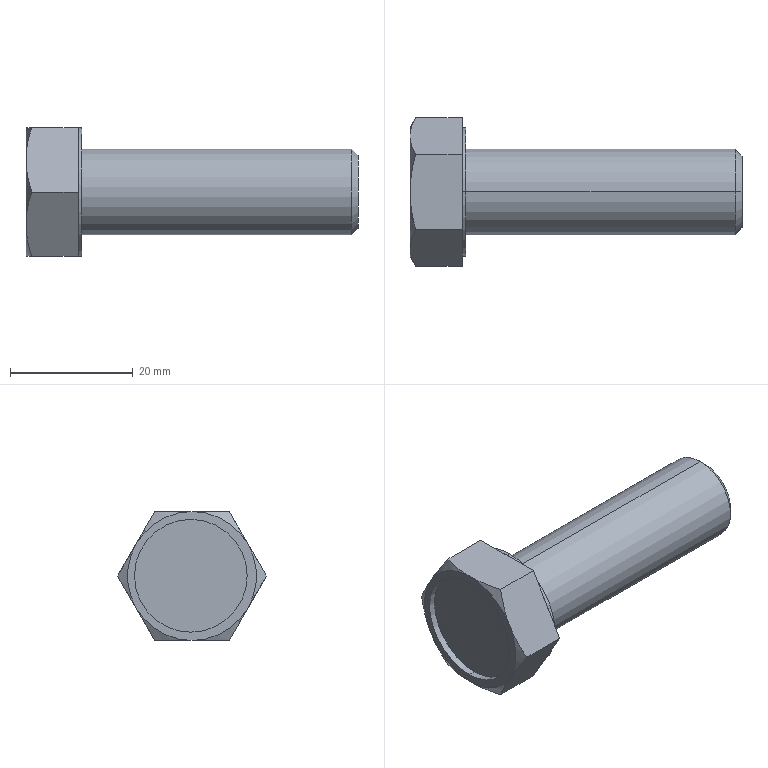Part | STEP file | formed hex screw_am_B18.2.3.2M - Formed hex screw, M14 x 2.0 x 45 --45WN | 1 solid | 30 faces | box 54.09 x 24.249 x 21 mm | volume 10041 mm3 | plane 16 | cone 8 | cylinder 6 | commonest cylinder face diameters 14 x2 18.375 x2 21 x2